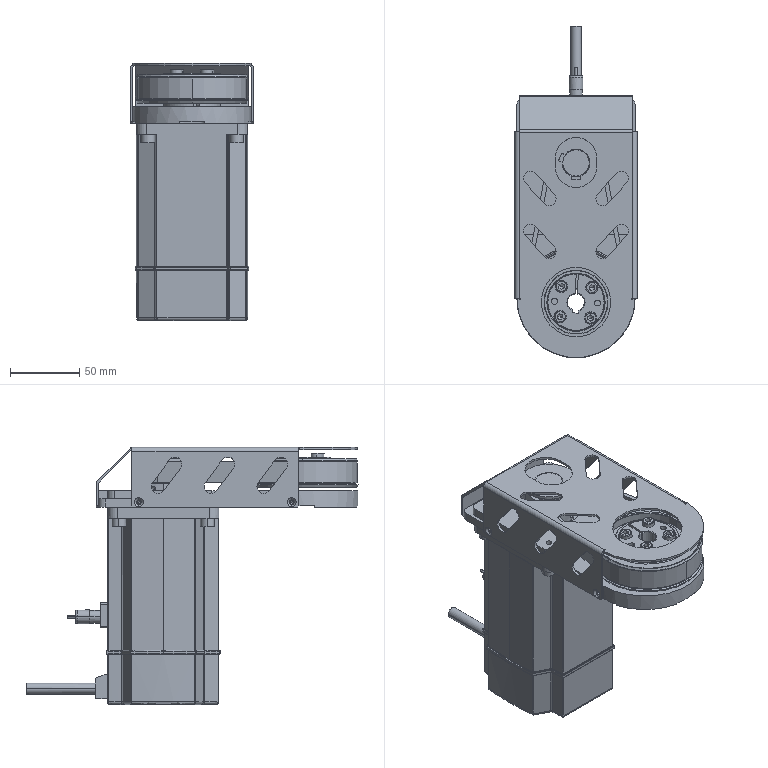Part | STEP file | Copy of CZ013-750W side link 2:1(K60)^K50A-1H20-S(formula driven)-L300-motor left- | 12 solids | 1406 faces | box 88 x 238.88 x 185 mm | volume 1086886 mm3 | cylinder 928 | plane 295 | cone 108 | spline 74 | torus 1 | commonest cylinder face diameters 0.6 x298 1.82 x177 75.66 x81 10 x52 1 x40 37.4 x40